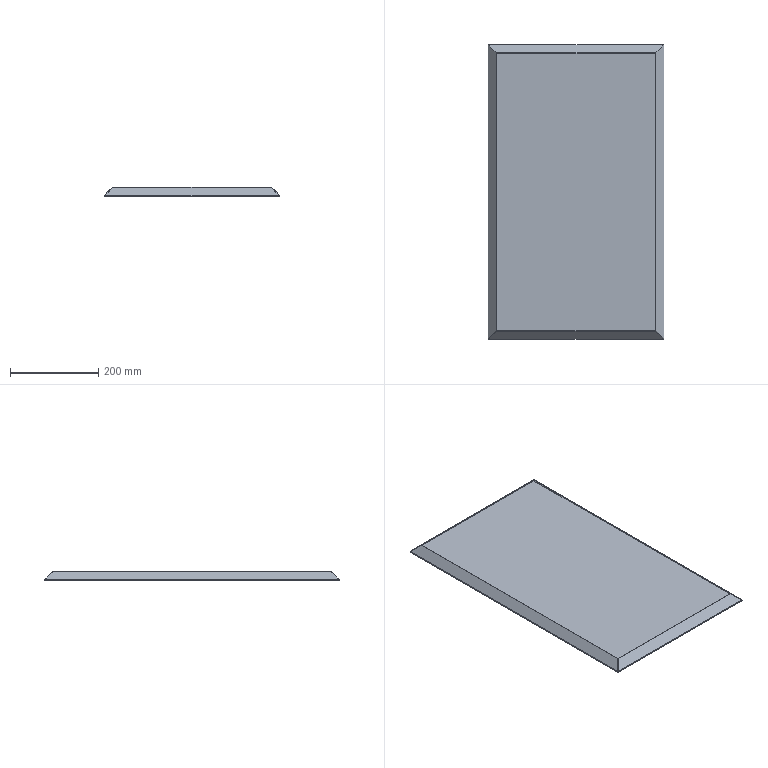Part | 1 solid | 50 faces | box 399.522 x 669.522 x 21.213 mm | volume 386480 mm3 | plane 22 | cylinder 16 | spline 12 | commonest cylinder face diameters 1.473 x8 3.873 x8